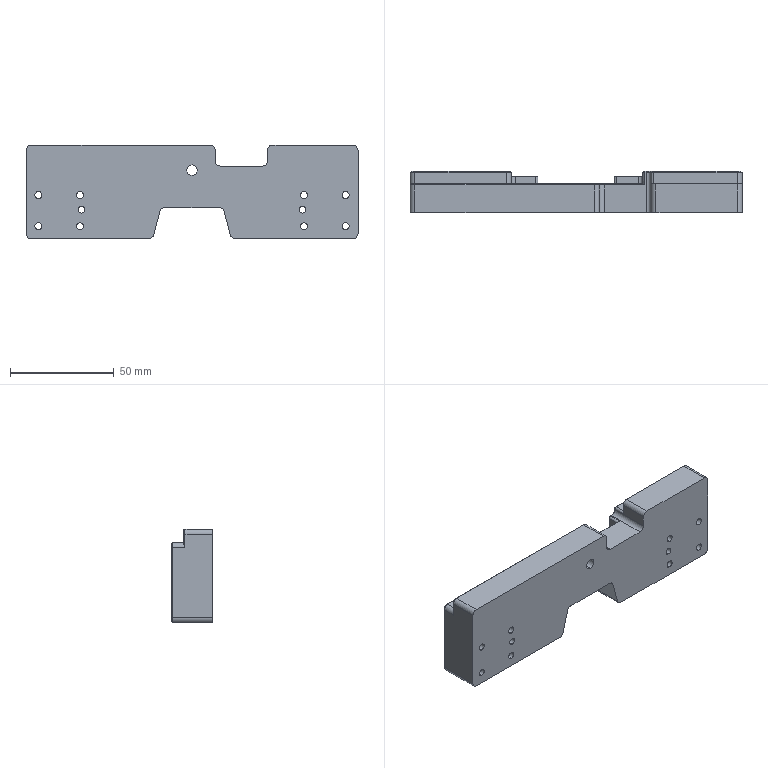Part | SolidWorks | features Cut 7, ICE 3, Fillet 2, HoleWzd 2, Chamfer 1, Extrusion 1 | 1 solid | 162 faces | box 160 x 20 x 45 mm | volume 104785 mm3 | cylinder 79 | plane 64 | cone 19 | commonest cylinder face diameters 4.6 x19 3.4 x16 6.5 x16 3.5 x6 2 x4 2.2 x4